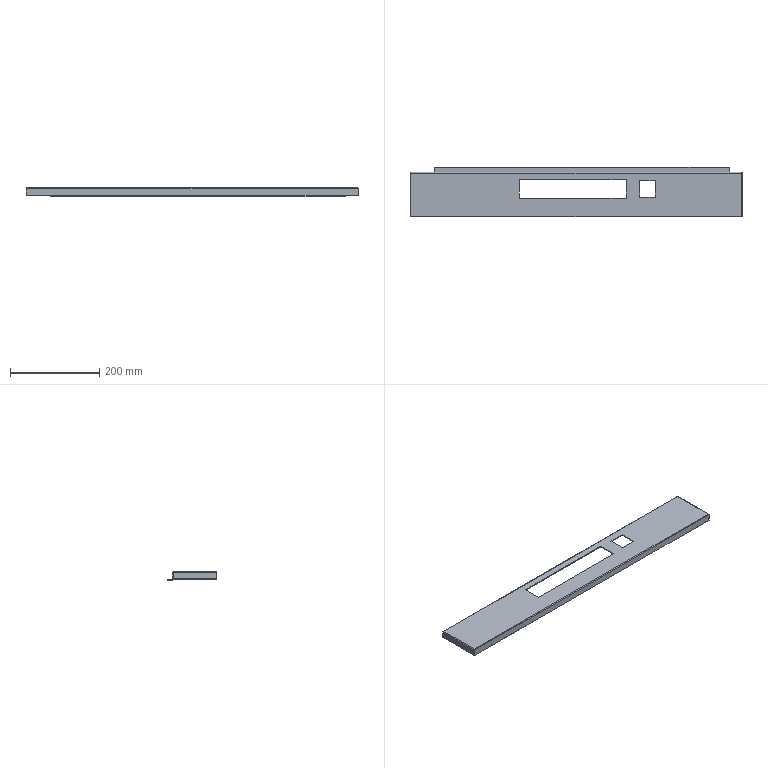Part | NX | features BREP 3 | 3 solids | 98 faces | box 745 x 112 x 18 mm | volume 155548 mm3 | plane 80 | cylinder 18 | commonest cylinder face diameters 0.02 x7 3.02 x7 3.3 x4